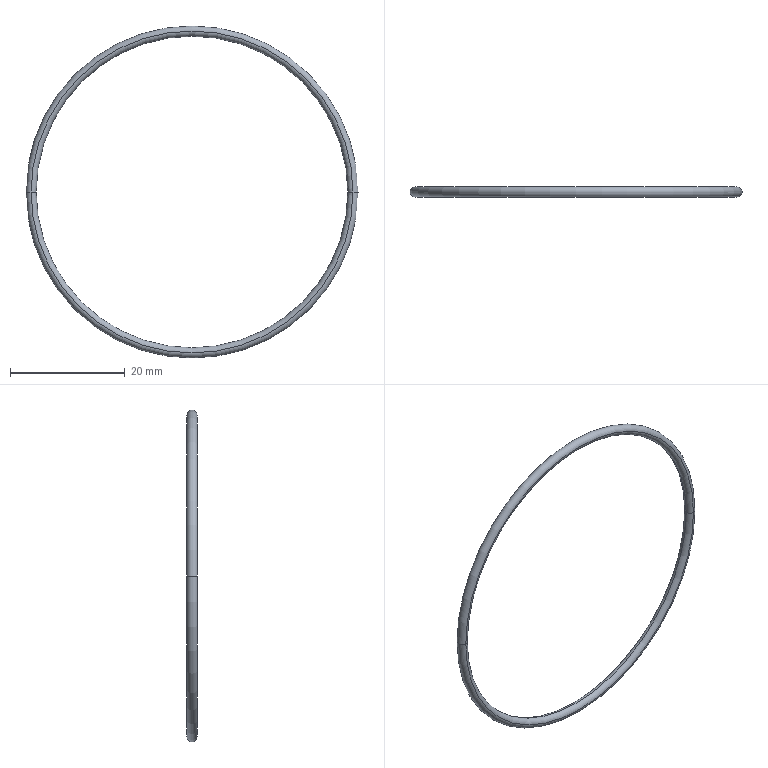Part | SolidWorks | features BaseBody 1 | 1 solid | 6 faces | box 57.96 x 1.78 x 57.96 mm | volume 439.199 mm3 | torus 6
STEP:
#1=CARTESIAN_POINT('',(1924.91,-273.38,853.));
#2=VERTEX_POINT('',#1);
#3=CARTESIAN_POINT('',(1925.8,-272.49,853.));
#4=VERTEX_POINT('',#3);
#5=CARTESIAN_POINT('',(1924.91,-272.49,853.));
#6=DIRECTION('',(0.,0.,1.));
#7=DIRECTION('',(0.,-1.,0.));
#8=AXIS2_PLACEMENT_3D('',#5,#6,#7);
#9=CIRCLE('',#8,0.89);
#10=EDGE_CURVE('',#2,#4,#9,.T.);
#11=ORIENTED_EDGE('',*,*,#10,.T.);
#12=CARTESIAN_POINT('',(1980.2,-272.49,853.));
#13=VERTEX_POINT('',#12);
#14=CARTESIAN_POINT('',(1953.,-272.49,853.));
#15=DIRECTION('',(0.,1.,0.));
#16=DIRECTION('',(-1.,0.,0.));
#17=AXIS2_PLACEMENT_3D('',#14,#15,#16);
#18=CIRCLE('',#17,27.2);
#19=EDGE_CURVE('',#4,#13,#18,.T.);
#20=ORIENTED_EDGE('',*,*,#19,.T.);
#21=CARTESIAN_POINT('',(1981.09,-273.38,853.));
#22=VERTEX_POINT('',#21);
#23=CARTESIAN_POINT('',(1981.09,-272.49,853.));
#24=DIRECTION('',(0.,0.,1.));
#25=DIRECTION('',(0.,-1.,0.));
#26=AXIS2_PLACEMENT_3D('',#23,#24,#25);
#27=CIRCLE('',#26,0.89);
#28=EDGE_CURVE('',#13,#22,#27,.T.);
#29=ORIENTED_EDGE('',*,*,#28,.T.);
#30=CARTESIAN_POINT('',(1953.,-273.38,853.));
#31=DIRECTION('',(0.,-1.,0.));
#32=DIRECTION('',(1.,0.,0.));
#33=AXIS2_PLACEMENT_3D('',#30,#31,#32);
#34=CIRCLE('',#33,28.09);
#35=EDGE_CURVE('',#22,#2,#34,.T.);
#36=ORIENTED_EDGE('',*,*,#35,.T.);
#37=EDGE_LOOP('',(#11,#20,#29,#36));
#38=FACE_OUTER_BOUND('',#37,.T.);
#39=CARTESIAN_POINT('',(1953.,-272.49,853.));
#40=DIRECTION('',(0.,1.,0.));
#41=DIRECTION('',(1.,0.,0.));
#42=AXIS2_PLACEMENT_3D('',#39,#40,#41);
#43=TOROIDAL_SURFACE('',#42,28.09,0.89);
#44=ADVANCED_FACE('',(#38),#43,.T.);
#45=ORIENTED_EDGE('',*,*,#28,.F.);
#46=CARTESIAN_POINT('',(1953.,-272.49,853.));
#47=DIRECTION('',(0.,1.,0.));
#48=DIRECTION('',(-1.,0.,0.));
#49=AXIS2_PLACEMENT_3D('',#46,#47,#48);
#50=CIRCLE('',#49,27.2);
#51=EDGE_CURVE('',#13,#4,#50,.T.);
#52=ORIENTED_EDGE('',*,*,#51,.T.);
#53=ORIENTED_EDGE('',*,*,#10,.F.);
#54=CARTESIAN_POINT('',(1953.,-273.38,853.));
#55=DIRECTION('',(0.,-1.,0.));
#56=DIRECTION('',(1.,0.,0.));
#57=AXIS2_PLACEMENT_3D('',#54,#55,#56);
#58=CIRCLE('',#57,28.09);
#59=EDGE_CURVE('',#2,#22,#58,.T.);
#60=ORIENTED_EDGE('',*,*,#59,.T.);
#61=EDGE_LOOP('',(#45,#52,#53,#60));
#62=FACE_OUTER_BOUND('',#61,.T.);
#63=CARTESIAN_POINT('',(1953.,-272.49,853.));
#64=DIRECTION('',(0.,1.,0.));
#65=DIRECTION('',(1.,0.,0.));
#66=AXIS2_PLACEMENT_3D('',#63,#64,#65);
#67=TOROIDAL_SURFACE('',#66,28.09,0.89);
#68=ADVANCED_FACE('',(#62),#67,.T.);
#69=ORIENTED_EDGE('',*,*,#35,.F.);
#70=CARTESIAN_POINT('',(1981.09,-271.6,853.));
#71=VERTEX_POINT('',#70);
#72=CARTESIAN_POINT('',(1981.09,-272.49,853.));
#73=DIRECTION('',(0.,0.,1.));
#74=DIRECTION('',(0.,1.,0.));
#75=AXIS2_PLACEMENT_3D('',#72,#73,#74);
#76=CIRCLE('',#75,0.89);
#77=EDGE_CURVE('',#22,#71,#76,.T.);
#78=ORIENTED_EDGE('',*,*,#77,.T.);
#79=CARTESIAN_POINT('',(1924.91,-271.6,853.));
#80=VERTEX_POINT('',#79);
#81=CARTESIAN_POINT('',(1953.,-271.6,853.));
#82=DIRECTION('',(0.,1.,0.));
#83=DIRECTION('',(1.,0.,0.));
#84=AXIS2_PLACEMENT_3D('',#81,#82,#83);
#85=CIRCLE('',#84,28.09);
#86=EDGE_CURVE('',#80,#71,#85,.T.);
#87=ORIENTED_EDGE('',*,*,#86,.F.);
#88=CARTESIAN_POINT('',(1924.91,-272.49,853.));
#89=DIRECTION('',(0.,0.,1.));
#90=DIRECTION('',(0.,1.,0.));
#91=AXIS2_PLACEMENT_3D('',#88,#89,#90);
#92=CIRCLE('',#91,0.89);
#93=EDGE_CURVE('',#80,#2,#92,.T.);
#94=ORIENTED_EDGE('',*,*,#93,.T.);
#95=EDGE_LOOP('',(#69,#78,#87,#94));
#96=FACE_OUTER_BOUND('',#95,.T.);
#97=CARTESIAN_POINT('',(1953.,-272.49,853.));
#98=DIRECTION('',(0.,1.,0.));
#99=DIRECTION('',(1.,0.,0.));
#100=AXIS2_PLACEMENT_3D('',#97,#98,#99);
#101=TOROIDAL_SURFACE('',#100,28.09,0.89);
#102=ADVANCED_FACE('',(#96),#101,.T.);
#103=CARTESIAN_POINT('',(1953.,-271.6,853.));
#104=DIRECTION('',(0.,1.,0.));
#105=DIRECTION('',(1.,0.,0.));
#106=AXIS2_PLACEMENT_3D('',#103,#104,#105);
#107=CIRCLE('',#106,28.09);
#108=EDGE_CURVE('',#71,#80,#107,.T.);
#109=ORIENTED_EDGE('',*,*,#108,.F.);
#110=ORIENTED_EDGE('',*,*,#77,.F.);
#111=ORIENTED_EDGE('',*,*,#59,.F.);
#112=ORIENTED_EDGE('',*,*,#93,.F.);
#113=EDGE_LOOP('',(#109,#110,#111,#112));
#114=FACE_OUTER_BOUND('',#113,.T.);
#115=CARTESIAN_POINT('',(1953.,-272.49,853.));
#116=DIRECTION('',(0.,1.,0.));
#117=DIRECTION('',(1.,0.,0.));
#118=AXIS2_PLACEMENT_3D('',#115,#116,#117);
#119=TOROIDAL_SURFACE('',#118,28.09,0.89);
#120=ADVANCED_FACE('',(#114),#119,.T.);
#121=ORIENTED_EDGE('',*,*,#51,.F.);
#122=CARTESIAN_POINT('',(1981.09,-272.49,853.));
#123=DIRECTION('',(0.,0.,1.));
#124=DIRECTION('',(0.,-1.,0.));
#125=AXIS2_PLACEMENT_3D('',#122,#123,#124);
#126=CIRCLE('',#125,0.89);
#127=EDGE_CURVE('',#71,#13,#126,.T.);
#128=ORIENTED_EDGE('',*,*,#127,.F.);
#129=ORIENTED_EDGE('',*,*,#108,.T.);
#130=CARTESIAN_POINT('',(1924.91,-272.49,853.));
#131=DIRECTION('',(0.,0.,1.));
#132=DIRECTION('',(0.,-1.,0.));
#133=AXIS2_PLACEMENT_3D('',#130,#131,#132);
#134=CIRCLE('',#133,0.89);
#135=EDGE_CURVE('',#4,#80,#134,.T.);
#136=ORIENTED_EDGE('',*,*,#135,.F.);
#137=EDGE_LOOP('',(#121,#128,#129,#136));
#138=FACE_OUTER_BOUND('',#137,.T.);
#139=CARTESIAN_POINT('',(1953.,-272.49,853.));
#140=DIRECTION('',(0.,1.,0.));
#141=DIRECTION('',(1.,0.,0.));
#142=AXIS2_PLACEMENT_3D('',#139,#140,#141);
#143=TOROIDAL_SURFACE('',#142,28.09,0.89);
#144=ADVANCED_FACE('',(#138),#143,.T.);
#145=ORIENTED_EDGE('',*,*,#19,.F.);
#146=ORIENTED_EDGE('',*,*,#135,.T.);
#147=ORIENTED_EDGE('',*,*,#86,.T.);
#148=ORIENTED_EDGE('',*,*,#127,.T.);
#149=EDGE_LOOP('',(#145,#146,#147,#148));
#150=FACE_OUTER_BOUND('',#149,.T.);
#151=CARTESIAN_POINT('',(1953.,-272.49,853.));
#152=DIRECTION('',(0.,1.,0.));
#153=DIRECTION('',(1.,0.,0.));
#154=AXIS2_PLACEMENT_3D('',#151,#152,#153);
#155=TOROIDAL_SURFACE('',#154,28.09,0.89);
#156=ADVANCED_FACE('',(#150),#155,.T.);
#157=CLOSED_SHELL('',(#44,#68,#102,#120,#144,#156));
#158=MANIFOLD_SOLID_BREP('',#157);
#159=CARTESIAN_POINT('',(0.,0.,0.));
#160=DIRECTION('',(0.,0.,1.));
#161=DIRECTION('',(1.,0.,0.));
#162=AXIS2_PLACEMENT_3D('',#159,#160,#161);
#163=(LENGTH_UNIT()NAMED_UNIT(*)SI_UNIT(.MILLI.,.METRE.));
#164=UNCERTAINTY_MEASURE_WITH_UNIT(LENGTH_MEASURE(0.00001),#163,'','');
#165=(NAMED_UNIT(*)PLANE_ANGLE_UNIT()SI_UNIT($,.RADIAN.));
#166=(NAMED_UNIT(*)SI_UNIT($,.STERADIAN.)SOLID_ANGLE_UNIT());
#167=(GEOMETRIC_REPRESENTATION_CONTEXT(3)GLOBAL_UNCERTAINTY_ASSIGNED_CONTEXT((#164))GLOBAL_UNIT_ASSIGNED_CONTEXT((#163,#165,#166))REPRESENTATION_CONTEXT('',''));
#168=ADVANCED_BREP_SHAPE_REPRESENTATION('',(#158,#162),#167);